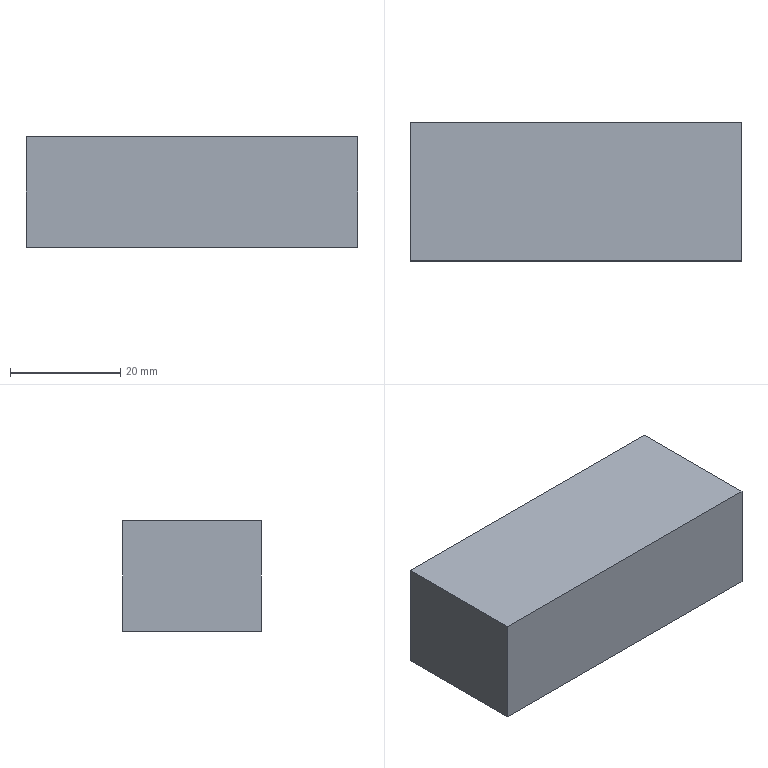Part | STEP file | 750078423 | 1 solid | 6 faces | box 60 x 25 x 20 mm | volume 30000 mm3 | plane 6
STEP:
#1=CARTESIAN_POINT('',(30.,25.,20.));
#2=VERTEX_POINT('',#1);
#3=CARTESIAN_POINT('',(30.,0.,20.));
#4=VERTEX_POINT('',#3);
#5=CARTESIAN_POINT('',(30.,0.,20.));
#6=DIRECTION('',(0.,-1.,0.));
#7=VECTOR('',#6,1000.);
#8=LINE('',#5,#7);
#9=EDGE_CURVE('',#2,#4,#8,.T.);
#10=ORIENTED_EDGE('',*,*,#9,.F.);
#11=CARTESIAN_POINT('',(-30.,25.,20.));
#12=VERTEX_POINT('',#11);
#13=CARTESIAN_POINT('',(0.,25.,20.));
#14=DIRECTION('',(1.,0.,0.));
#15=VECTOR('',#14,1000.);
#16=LINE('',#13,#15);
#17=EDGE_CURVE('',#12,#2,#16,.T.);
#18=ORIENTED_EDGE('',*,*,#17,.F.);
#19=CARTESIAN_POINT('',(-30.,0.,20.));
#20=VERTEX_POINT('',#19);
#21=CARTESIAN_POINT('',(-30.,0.,20.));
#22=DIRECTION('',(0.,1.,0.));
#23=VECTOR('',#22,1000.);
#24=LINE('',#21,#23);
#25=EDGE_CURVE('',#20,#12,#24,.T.);
#26=ORIENTED_EDGE('',*,*,#25,.F.);
#27=CARTESIAN_POINT('',(0.,0.,20.));
#28=DIRECTION('',(-1.,0.,0.));
#29=VECTOR('',#28,1000.);
#30=LINE('',#27,#29);
#31=EDGE_CURVE('',#4,#20,#30,.T.);
#32=ORIENTED_EDGE('',*,*,#31,.F.);
#33=EDGE_LOOP('',(#10,#18,#26,#32));
#34=FACE_OUTER_BOUND('',#33,.T.);
#35=CARTESIAN_POINT('',(0.,0.,20.));
#36=DIRECTION('',(0.,0.,-1.));
#37=DIRECTION('',(-1.,0.,0.));
#38=AXIS2_PLACEMENT_3D('',#35,#36,#37);
#39=PLANE('',#38);
#40=ADVANCED_FACE('',(#34),#39,.F.);
#41=ORIENTED_EDGE('',*,*,#31,.T.);
#42=CARTESIAN_POINT('',(-30.,0.,0.));
#43=VERTEX_POINT('',#42);
#44=CARTESIAN_POINT('',(-30.,0.,20.));
#45=DIRECTION('',(0.,0.,-1.));
#46=VECTOR('',#45,1000.);
#47=LINE('',#44,#46);
#48=EDGE_CURVE('',#20,#43,#47,.T.);
#49=ORIENTED_EDGE('',*,*,#48,.T.);
#50=CARTESIAN_POINT('',(30.,0.,0.));
#51=VERTEX_POINT('',#50);
#52=CARTESIAN_POINT('',(30.,0.,0.));
#53=DIRECTION('',(1.,0.,0.));
#54=VECTOR('',#53,1000.);
#55=LINE('',#52,#54);
#56=EDGE_CURVE('',#43,#51,#55,.T.);
#57=ORIENTED_EDGE('',*,*,#56,.T.);
#58=CARTESIAN_POINT('',(30.,0.,20.));
#59=DIRECTION('',(0.,0.,1.));
#60=VECTOR('',#59,1000.);
#61=LINE('',#58,#60);
#62=EDGE_CURVE('',#51,#4,#61,.T.);
#63=ORIENTED_EDGE('',*,*,#62,.T.);
#64=EDGE_LOOP('',(#41,#49,#57,#63));
#65=FACE_OUTER_BOUND('',#64,.T.);
#66=CARTESIAN_POINT('',(30.,0.,20.));
#67=DIRECTION('',(0.,-1.,0.));
#68=DIRECTION('',(1.,0.,0.));
#69=AXIS2_PLACEMENT_3D('',#66,#67,#68);
#70=PLANE('',#69);
#71=ADVANCED_FACE('',(#65),#70,.T.);
#72=ORIENTED_EDGE('',*,*,#9,.T.);
#73=ORIENTED_EDGE('',*,*,#62,.F.);
#74=CARTESIAN_POINT('',(30.,25.,0.));
#75=VERTEX_POINT('',#74);
#76=CARTESIAN_POINT('',(30.,25.,0.));
#77=DIRECTION('',(0.,1.,0.));
#78=VECTOR('',#77,1000.);
#79=LINE('',#76,#78);
#80=EDGE_CURVE('',#51,#75,#79,.T.);
#81=ORIENTED_EDGE('',*,*,#80,.T.);
#82=CARTESIAN_POINT('',(30.,25.,20.));
#83=DIRECTION('',(0.,0.,1.));
#84=VECTOR('',#83,1000.);
#85=LINE('',#82,#84);
#86=EDGE_CURVE('',#75,#2,#85,.T.);
#87=ORIENTED_EDGE('',*,*,#86,.T.);
#88=EDGE_LOOP('',(#72,#73,#81,#87));
#89=FACE_OUTER_BOUND('',#88,.T.);
#90=CARTESIAN_POINT('',(30.,25.,20.));
#91=DIRECTION('',(1.,0.,0.));
#92=DIRECTION('',(0.,1.,0.));
#93=AXIS2_PLACEMENT_3D('',#90,#91,#92);
#94=PLANE('',#93);
#95=ADVANCED_FACE('',(#89),#94,.T.);
#96=ORIENTED_EDGE('',*,*,#17,.T.);
#97=ORIENTED_EDGE('',*,*,#86,.F.);
#98=CARTESIAN_POINT('',(-30.,25.,0.));
#99=VERTEX_POINT('',#98);
#100=CARTESIAN_POINT('',(-30.,25.,0.));
#101=DIRECTION('',(-1.,0.,0.));
#102=VECTOR('',#101,1000.);
#103=LINE('',#100,#102);
#104=EDGE_CURVE('',#75,#99,#103,.T.);
#105=ORIENTED_EDGE('',*,*,#104,.T.);
#106=CARTESIAN_POINT('',(-30.,25.,20.));
#107=DIRECTION('',(0.,0.,1.));
#108=VECTOR('',#107,1000.);
#109=LINE('',#106,#108);
#110=EDGE_CURVE('',#99,#12,#109,.T.);
#111=ORIENTED_EDGE('',*,*,#110,.T.);
#112=EDGE_LOOP('',(#96,#97,#105,#111));
#113=FACE_OUTER_BOUND('',#112,.T.);
#114=CARTESIAN_POINT('',(-30.,25.,20.));
#115=DIRECTION('',(0.,1.,0.));
#116=DIRECTION('',(0.,0.,1.));
#117=AXIS2_PLACEMENT_3D('',#114,#115,#116);
#118=PLANE('',#117);
#119=ADVANCED_FACE('',(#113),#118,.T.);
#120=ORIENTED_EDGE('',*,*,#25,.T.);
#121=ORIENTED_EDGE('',*,*,#110,.F.);
#122=CARTESIAN_POINT('',(-30.,0.,0.));
#123=DIRECTION('',(0.,-1.,0.));
#124=VECTOR('',#123,1000.);
#125=LINE('',#122,#124);
#126=EDGE_CURVE('',#99,#43,#125,.T.);
#127=ORIENTED_EDGE('',*,*,#126,.T.);
#128=ORIENTED_EDGE('',*,*,#48,.F.);
#129=EDGE_LOOP('',(#120,#121,#127,#128));
#130=FACE_OUTER_BOUND('',#129,.T.);
#131=CARTESIAN_POINT('',(-30.,0.,20.));
#132=DIRECTION('',(-1.,0.,0.));
#133=DIRECTION('',(0.,-1.,0.));
#134=AXIS2_PLACEMENT_3D('',#131,#132,#133);
#135=PLANE('',#134);
#136=ADVANCED_FACE('',(#130),#135,.T.);
#137=ORIENTED_EDGE('',*,*,#104,.F.);
#138=ORIENTED_EDGE('',*,*,#80,.F.);
#139=ORIENTED_EDGE('',*,*,#56,.F.);
#140=ORIENTED_EDGE('',*,*,#126,.F.);
#141=EDGE_LOOP('',(#137,#138,#139,#140));
#142=FACE_OUTER_BOUND('',#141,.T.);
#143=CARTESIAN_POINT('',(0.,0.,0.));
#144=DIRECTION('',(0.,0.,-1.));
#145=DIRECTION('',(-1.,0.,0.));
#146=AXIS2_PLACEMENT_3D('',#143,#144,#145);
#147=PLANE('',#146);
#148=ADVANCED_FACE('',(#142),#147,.T.);
#149=CLOSED_SHELL('',(#40,#71,#95,#119,#136,#148));
#150=MANIFOLD_SOLID_BREP('',#149);
#151=CARTESIAN_POINT('',(0.,0.,0.));
#152=DIRECTION('',(0.,0.,1.));
#153=DIRECTION('',(1.,0.,0.));
#154=AXIS2_PLACEMENT_3D('',#151,#152,#153);
#155=(LENGTH_UNIT()NAMED_UNIT(*)SI_UNIT(.MILLI.,.METRE.));
#156=UNCERTAINTY_MEASURE_WITH_UNIT(LENGTH_MEASURE(0.00001),#155,'','');
#157=(NAMED_UNIT(*)PLANE_ANGLE_UNIT()SI_UNIT($,.RADIAN.));
#158=(NAMED_UNIT(*)SI_UNIT($,.STERADIAN.)SOLID_ANGLE_UNIT());
#159=(GEOMETRIC_REPRESENTATION_CONTEXT(3)GLOBAL_UNCERTAINTY_ASSIGNED_CONTEXT((#156))GLOBAL_UNIT_ASSIGNED_CONTEXT((#155,#157,#158))REPRESENTATION_CONTEXT('',''));
#160=ADVANCED_BREP_SHAPE_REPRESENTATION('',(#150,#154),#159);